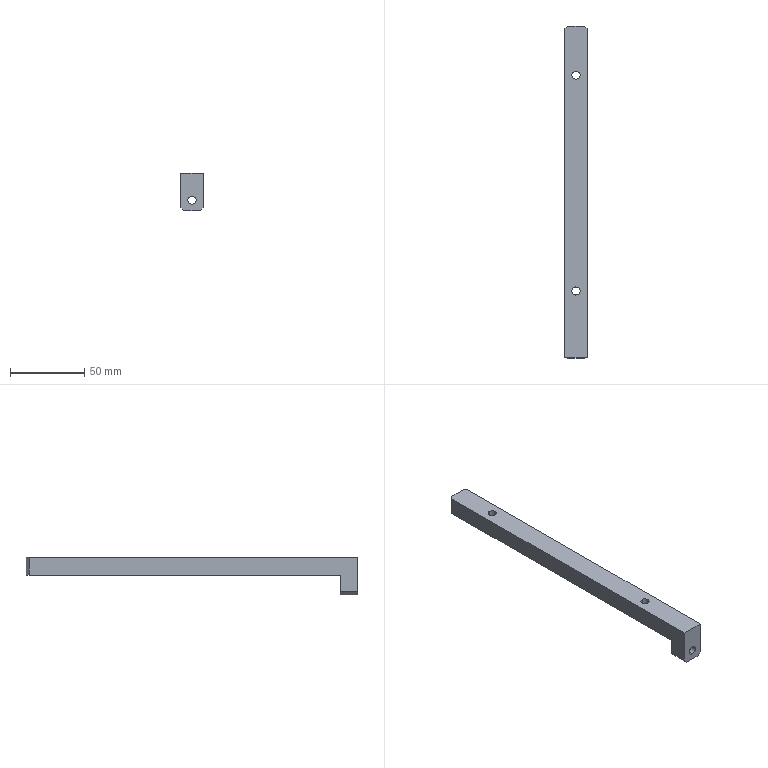Part | SolidWorks | features HoleWzd 2, Chamfer 1, Extrusion 1 | 1 solid | 24 faces | box 15 x 223.1 x 25 mm | volume 40922 mm3 | plane 14 | cylinder 10 | commonest cylinder face diameters 5.5 x6 10 x4
STEP:
#1=CARTESIAN_POINT('',(7.5,12.,-15.25));
#2=VERTEX_POINT('',#1);
#3=CARTESIAN_POINT('',(7.5,12.,-20.75));
#4=VERTEX_POINT('',#3);
#5=CARTESIAN_POINT('',(7.5,12.,-18.));
#6=DIRECTION('',(0.,-1.,0.));
#7=DIRECTION('',(0.,0.,-1.));
#8=AXIS2_PLACEMENT_3D('',#5,#6,#7);
#9=CIRCLE('',#8,2.75);
#10=EDGE_CURVE('',#2,#4,#9,.T.);
#11=ORIENTED_EDGE('',*,*,#10,.F.);
#12=CARTESIAN_POINT('',(7.5,0.,-15.25));
#13=VERTEX_POINT('',#12);
#14=CARTESIAN_POINT('',(7.5,0.,-15.25));
#15=DIRECTION('',(0.,-1.,0.));
#16=VECTOR('',#15,1000.);
#17=LINE('',#14,#16);
#18=EDGE_CURVE('',#2,#13,#17,.T.);
#19=ORIENTED_EDGE('',*,*,#18,.T.);
#20=CARTESIAN_POINT('',(7.5,0.,-20.75));
#21=VERTEX_POINT('',#20);
#22=CARTESIAN_POINT('',(7.5,0.,-18.));
#23=DIRECTION('',(0.,-1.,0.));
#24=DIRECTION('',(0.,0.,-1.));
#25=AXIS2_PLACEMENT_3D('',#22,#23,#24);
#26=CIRCLE('',#25,2.75);
#27=EDGE_CURVE('',#13,#21,#26,.T.);
#28=ORIENTED_EDGE('',*,*,#27,.T.);
#29=CARTESIAN_POINT('',(7.5,0.,-20.75));
#30=DIRECTION('',(0.,-1.,0.));
#31=VECTOR('',#30,1000.);
#32=LINE('',#29,#31);
#33=EDGE_CURVE('',#4,#21,#32,.T.);
#34=ORIENTED_EDGE('',*,*,#33,.F.);
#35=EDGE_LOOP('',(#11,#19,#28,#34));
#36=FACE_OUTER_BOUND('',#35,.T.);
#37=CARTESIAN_POINT('',(7.5,0.,-18.));
#38=DIRECTION('',(0.,-1.,0.));
#39=DIRECTION('',(0.,0.,-1.));
#40=AXIS2_PLACEMENT_3D('',#37,#38,#39);
#41=CYLINDRICAL_SURFACE('',#40,2.75);
#42=ADVANCED_FACE('',(#36),#41,.F.);
#43=CARTESIAN_POINT('',(7.5,185.,-6.3));
#44=VERTEX_POINT('',#43);
#45=CARTESIAN_POINT('',(7.5,195.,-6.3));
#46=VERTEX_POINT('',#45);
#47=CARTESIAN_POINT('',(7.5,190.,-6.3));
#48=DIRECTION('',(0.,0.,-1.));
#49=DIRECTION('',(0.,1.,0.));
#50=AXIS2_PLACEMENT_3D('',#47,#48,#49);
#51=CIRCLE('',#50,5.);
#52=EDGE_CURVE('',#44,#46,#51,.T.);
#53=ORIENTED_EDGE('',*,*,#52,.F.);
#54=CARTESIAN_POINT('',(7.5,185.,-12.));
#55=VERTEX_POINT('',#54);
#56=CARTESIAN_POINT('',(7.5,185.,-12.));
#57=DIRECTION('',(0.,0.,-1.));
#58=VECTOR('',#57,1000.);
#59=LINE('',#56,#58);
#60=EDGE_CURVE('',#44,#55,#59,.T.);
#61=ORIENTED_EDGE('',*,*,#60,.T.);
#62=CARTESIAN_POINT('',(7.5,195.,-12.));
#63=VERTEX_POINT('',#62);
#64=CARTESIAN_POINT('',(7.5,190.,-12.));
#65=DIRECTION('',(0.,0.,-1.));
#66=DIRECTION('',(0.,1.,0.));
#67=AXIS2_PLACEMENT_3D('',#64,#65,#66);
#68=CIRCLE('',#67,5.);
#69=EDGE_CURVE('',#55,#63,#68,.T.);
#70=ORIENTED_EDGE('',*,*,#69,.T.);
#71=CARTESIAN_POINT('',(7.5,195.,-12.));
#72=DIRECTION('',(0.,0.,-1.));
#73=VECTOR('',#72,1000.);
#74=LINE('',#71,#73);
#75=EDGE_CURVE('',#46,#63,#74,.T.);
#76=ORIENTED_EDGE('',*,*,#75,.F.);
#77=EDGE_LOOP('',(#53,#61,#70,#76));
#78=FACE_OUTER_BOUND('',#77,.T.);
#79=CARTESIAN_POINT('',(7.5,190.,-12.));
#80=DIRECTION('',(0.,0.,-1.));
#81=DIRECTION('',(0.,1.,0.));
#82=AXIS2_PLACEMENT_3D('',#79,#80,#81);
#83=CYLINDRICAL_SURFACE('',#82,5.);
#84=ADVANCED_FACE('',(#78),#83,.F.);
#85=CARTESIAN_POINT('',(7.5,187.25,0.));
#86=VERTEX_POINT('',#85);
#87=CARTESIAN_POINT('',(7.5,192.75,0.));
#88=VERTEX_POINT('',#87);
#89=CARTESIAN_POINT('',(7.5,190.,0.));
#90=DIRECTION('',(0.,0.,-1.));
#91=DIRECTION('',(0.,1.,0.));
#92=AXIS2_PLACEMENT_3D('',#89,#90,#91);
#93=CIRCLE('',#92,2.75);
#94=EDGE_CURVE('',#86,#88,#93,.T.);
#95=ORIENTED_EDGE('',*,*,#94,.F.);
#96=CARTESIAN_POINT('',(7.5,187.25,-6.3));
#97=VERTEX_POINT('',#96);
#98=CARTESIAN_POINT('',(7.5,187.25,-12.));
#99=DIRECTION('',(0.,0.,-1.));
#100=VECTOR('',#99,1000.);
#101=LINE('',#98,#100);
#102=EDGE_CURVE('',#86,#97,#101,.T.);
#103=ORIENTED_EDGE('',*,*,#102,.T.);
#104=CARTESIAN_POINT('',(7.5,192.75,-6.3));
#105=VERTEX_POINT('',#104);
#106=CARTESIAN_POINT('',(7.5,190.,-6.3));
#107=DIRECTION('',(0.,0.,-1.));
#108=DIRECTION('',(0.,1.,0.));
#109=AXIS2_PLACEMENT_3D('',#106,#107,#108);
#110=CIRCLE('',#109,2.75);
#111=EDGE_CURVE('',#97,#105,#110,.T.);
#112=ORIENTED_EDGE('',*,*,#111,.T.);
#113=CARTESIAN_POINT('',(7.5,192.75,-12.));
#114=DIRECTION('',(0.,0.,-1.));
#115=VECTOR('',#114,1000.);
#116=LINE('',#113,#115);
#117=EDGE_CURVE('',#88,#105,#116,.T.);
#118=ORIENTED_EDGE('',*,*,#117,.F.);
#119=EDGE_LOOP('',(#95,#103,#112,#118));
#120=FACE_OUTER_BOUND('',#119,.T.);
#121=CARTESIAN_POINT('',(7.5,190.,-12.));
#122=DIRECTION('',(0.,0.,-1.));
#123=DIRECTION('',(0.,1.,0.));
#124=AXIS2_PLACEMENT_3D('',#121,#122,#123);
#125=CYLINDRICAL_SURFACE('',#124,2.75);
#126=ADVANCED_FACE('',(#120),#125,.F.);
#127=CARTESIAN_POINT('',(7.5,40.,-6.3));
#128=VERTEX_POINT('',#127);
#129=CARTESIAN_POINT('',(7.5,50.,-6.3));
#130=VERTEX_POINT('',#129);
#131=CARTESIAN_POINT('',(7.5,45.,-6.3));
#132=DIRECTION('',(0.,0.,-1.));
#133=DIRECTION('',(0.,1.,0.));
#134=AXIS2_PLACEMENT_3D('',#131,#132,#133);
#135=CIRCLE('',#134,5.);
#136=EDGE_CURVE('',#128,#130,#135,.T.);
#137=ORIENTED_EDGE('',*,*,#136,.F.);
#138=CARTESIAN_POINT('',(7.5,40.,-12.));
#139=VERTEX_POINT('',#138);
#140=CARTESIAN_POINT('',(7.5,40.,-12.));
#141=DIRECTION('',(0.,0.,-1.));
#142=VECTOR('',#141,1000.);
#143=LINE('',#140,#142);
#144=EDGE_CURVE('',#128,#139,#143,.T.);
#145=ORIENTED_EDGE('',*,*,#144,.T.);
#146=CARTESIAN_POINT('',(7.5,50.,-12.));
#147=VERTEX_POINT('',#146);
#148=CARTESIAN_POINT('',(7.5,45.,-12.));
#149=DIRECTION('',(0.,0.,-1.));
#150=DIRECTION('',(0.,1.,0.));
#151=AXIS2_PLACEMENT_3D('',#148,#149,#150);
#152=CIRCLE('',#151,5.);
#153=EDGE_CURVE('',#139,#147,#152,.T.);
#154=ORIENTED_EDGE('',*,*,#153,.T.);
#155=CARTESIAN_POINT('',(7.5,50.,-12.));
#156=DIRECTION('',(0.,0.,-1.));
#157=VECTOR('',#156,1000.);
#158=LINE('',#155,#157);
#159=EDGE_CURVE('',#130,#147,#158,.T.);
#160=ORIENTED_EDGE('',*,*,#159,.F.);
#161=EDGE_LOOP('',(#137,#145,#154,#160));
#162=FACE_OUTER_BOUND('',#161,.T.);
#163=CARTESIAN_POINT('',(7.5,45.,-12.));
#164=DIRECTION('',(0.,0.,-1.));
#165=DIRECTION('',(0.,1.,0.));
#166=AXIS2_PLACEMENT_3D('',#163,#164,#165);
#167=CYLINDRICAL_SURFACE('',#166,5.);
#168=ADVANCED_FACE('',(#162),#167,.F.);
#169=CARTESIAN_POINT('',(7.5,42.25,0.));
#170=VERTEX_POINT('',#169);
#171=CARTESIAN_POINT('',(7.5,47.75,0.));
#172=VERTEX_POINT('',#171);
#173=CARTESIAN_POINT('',(7.5,45.,0.));
#174=DIRECTION('',(0.,0.,-1.));
#175=DIRECTION('',(0.,1.,0.));
#176=AXIS2_PLACEMENT_3D('',#173,#174,#175);
#177=CIRCLE('',#176,2.75);
#178=EDGE_CURVE('',#170,#172,#177,.T.);
#179=ORIENTED_EDGE('',*,*,#178,.F.);
#180=CARTESIAN_POINT('',(7.5,42.25,-6.3));
#181=VERTEX_POINT('',#180);
#182=CARTESIAN_POINT('',(7.5,42.25,-12.));
#183=DIRECTION('',(0.,0.,-1.));
#184=VECTOR('',#183,1000.);
#185=LINE('',#182,#184);
#186=EDGE_CURVE('',#170,#181,#185,.T.);
#187=ORIENTED_EDGE('',*,*,#186,.T.);
#188=CARTESIAN_POINT('',(7.5,47.75,-6.3));
#189=VERTEX_POINT('',#188);
#190=CARTESIAN_POINT('',(7.5,45.,-6.3));
#191=DIRECTION('',(0.,0.,-1.));
#192=DIRECTION('',(0.,1.,0.));
#193=AXIS2_PLACEMENT_3D('',#190,#191,#192);
#194=CIRCLE('',#193,2.75);
#195=EDGE_CURVE('',#181,#189,#194,.T.);
#196=ORIENTED_EDGE('',*,*,#195,.T.);
#197=CARTESIAN_POINT('',(7.5,47.75,-12.));
#198=DIRECTION('',(0.,0.,-1.));
#199=VECTOR('',#198,1000.);
#200=LINE('',#197,#199);
#201=EDGE_CURVE('',#172,#189,#200,.T.);
#202=ORIENTED_EDGE('',*,*,#201,.F.);
#203=EDGE_LOOP('',(#179,#187,#196,#202));
#204=FACE_OUTER_BOUND('',#203,.T.);
#205=CARTESIAN_POINT('',(7.5,45.,-12.));
#206=DIRECTION('',(0.,0.,-1.));
#207=DIRECTION('',(0.,1.,0.));
#208=AXIS2_PLACEMENT_3D('',#205,#206,#207);
#209=CYLINDRICAL_SURFACE('',#208,2.75);
#210=ADVANCED_FACE('',(#204),#209,.F.);
#211=CARTESIAN_POINT('',(7.5,190.,0.));
#212=DIRECTION('',(0.,0.,-1.));
#213=DIRECTION('',(0.,1.,0.));
#214=AXIS2_PLACEMENT_3D('',#211,#212,#213);
#215=CIRCLE('',#214,2.75);
#216=EDGE_CURVE('',#88,#86,#215,.T.);
#217=ORIENTED_EDGE('',*,*,#216,.T.);
#218=ORIENTED_EDGE('',*,*,#94,.T.);
#219=EDGE_LOOP('',(#217,#218));
#220=FACE_BOUND('',#219,.T.);
#221=CARTESIAN_POINT('',(7.5,45.,0.));
#222=DIRECTION('',(0.,0.,-1.));
#223=DIRECTION('',(0.,1.,0.));
#224=AXIS2_PLACEMENT_3D('',#221,#222,#223);
#225=CIRCLE('',#224,2.75);
#226=EDGE_CURVE('',#172,#170,#225,.T.);
#227=ORIENTED_EDGE('',*,*,#226,.T.);
#228=ORIENTED_EDGE('',*,*,#178,.T.);
#229=EDGE_LOOP('',(#227,#228));
#230=FACE_BOUND('',#229,.T.);
#231=CARTESIAN_POINT('',(13.,223.1,0.));
#232=VERTEX_POINT('',#231);
#233=CARTESIAN_POINT('',(2.,223.1,0.));
#234=VERTEX_POINT('',#233);
#235=CARTESIAN_POINT('',(15.,223.1,0.));
#236=DIRECTION('',(-1.,0.,0.));
#237=VECTOR('',#236,1000.);
#238=LINE('',#235,#237);
#239=EDGE_CURVE('',#232,#234,#238,.T.);
#240=ORIENTED_EDGE('',*,*,#239,.T.);
#241=CARTESIAN_POINT('',(0.,221.1,0.));
#242=VERTEX_POINT('',#241);
#243=CARTESIAN_POINT('',(2.,223.1,0.));
#244=DIRECTION('',(-0.7071,-0.7071,0.));
#245=VECTOR('',#244,1000.);
#246=LINE('',#243,#245);
#247=EDGE_CURVE('',#234,#242,#246,.T.);
#248=ORIENTED_EDGE('',*,*,#247,.T.);
#249=CARTESIAN_POINT('',(0.,0.,0.));
#250=VERTEX_POINT('',#249);
#251=CARTESIAN_POINT('',(0.,223.1,0.));
#252=DIRECTION('',(0.,-1.,0.));
#253=VECTOR('',#252,1000.);
#254=LINE('',#251,#253);
#255=EDGE_CURVE('',#242,#250,#254,.T.);
#256=ORIENTED_EDGE('',*,*,#255,.T.);
#257=CARTESIAN_POINT('',(15.,0.,0.));
#258=VERTEX_POINT('',#257);
#259=CARTESIAN_POINT('',(15.,0.,0.));
#260=DIRECTION('',(-1.,0.,0.));
#261=VECTOR('',#260,1000.);
#262=LINE('',#259,#261);
#263=EDGE_CURVE('',#258,#250,#262,.T.);
#264=ORIENTED_EDGE('',*,*,#263,.F.);
#265=CARTESIAN_POINT('',(15.,221.1,0.));
#266=VERTEX_POINT('',#265);
#267=CARTESIAN_POINT('',(15.,223.1,0.));
#268=DIRECTION('',(0.,-1.,0.));
#269=VECTOR('',#268,1000.);
#270=LINE('',#267,#269);
#271=EDGE_CURVE('',#266,#258,#270,.T.);
#272=ORIENTED_EDGE('',*,*,#271,.F.);
#273=CARTESIAN_POINT('',(15.,221.1,0.));
#274=DIRECTION('',(-0.7071,0.7071,0.));
#275=VECTOR('',#274,1000.);
#276=LINE('',#273,#275);
#277=EDGE_CURVE('',#266,#232,#276,.T.);
#278=ORIENTED_EDGE('',*,*,#277,.T.);
#279=EDGE_LOOP('',(#240,#248,#256,#264,#272,#278));
#280=FACE_OUTER_BOUND('',#279,.T.);
#281=CARTESIAN_POINT('',(15.,223.1,0.));
#282=DIRECTION('',(0.,0.,-1.));
#283=DIRECTION('',(-1.,0.,0.));
#284=AXIS2_PLACEMENT_3D('',#281,#282,#283);
#285=PLANE('',#284);
#286=ADVANCED_FACE('',(#220,#230,#280),#285,.F.);
#287=CARTESIAN_POINT('',(7.5,0.,-18.));
#288=DIRECTION('',(0.,-1.,0.));
#289=DIRECTION('',(0.,0.,-1.));
#290=AXIS2_PLACEMENT_3D('',#287,#288,#289);
#291=CIRCLE('',#290,2.75);
#292=EDGE_CURVE('',#21,#13,#291,.T.);
#293=ORIENTED_EDGE('',*,*,#292,.F.);
#294=ORIENTED_EDGE('',*,*,#27,.F.);
#295=EDGE_LOOP('',(#293,#294));
#296=FACE_BOUND('',#295,.T.);
#297=CARTESIAN_POINT('',(0.,0.,-23.));
#298=VERTEX_POINT('',#297);
#299=CARTESIAN_POINT('',(0.,0.,0.));
#300=DIRECTION('',(0.,0.,-1.));
#301=VECTOR('',#300,1000.);
#302=LINE('',#299,#301);
#303=EDGE_CURVE('',#250,#298,#302,.T.);
#304=ORIENTED_EDGE('',*,*,#303,.T.);
#305=CARTESIAN_POINT('',(2.,0.,-25.));
#306=VERTEX_POINT('',#305);
#307=CARTESIAN_POINT('',(2.,0.,-25.));
#308=DIRECTION('',(0.7071,0.,-0.7071));
#309=VECTOR('',#308,1000.);
#310=LINE('',#307,#309);
#311=EDGE_CURVE('',#298,#306,#310,.T.);
#312=ORIENTED_EDGE('',*,*,#311,.T.);
#313=CARTESIAN_POINT('',(13.,0.,-25.));
#314=VERTEX_POINT('',#313);
#315=CARTESIAN_POINT('',(15.,0.,-25.));
#316=DIRECTION('',(-1.,0.,0.));
#317=VECTOR('',#316,1000.);
#318=LINE('',#315,#317);
#319=EDGE_CURVE('',#314,#306,#318,.T.);
#320=ORIENTED_EDGE('',*,*,#319,.F.);
#321=CARTESIAN_POINT('',(15.,0.,-23.));
#322=VERTEX_POINT('',#321);
#323=CARTESIAN_POINT('',(15.,0.,-23.));
#324=DIRECTION('',(0.7071,0.,0.7071));
#325=VECTOR('',#324,1000.);
#326=LINE('',#323,#325);
#327=EDGE_CURVE('',#314,#322,#326,.T.);
#328=ORIENTED_EDGE('',*,*,#327,.T.);
#329=CARTESIAN_POINT('',(15.,0.,0.));
#330=DIRECTION('',(0.,0.,-1.));
#331=VECTOR('',#330,1000.);
#332=LINE('',#329,#331);
#333=EDGE_CURVE('',#258,#322,#332,.T.);
#334=ORIENTED_EDGE('',*,*,#333,.F.);
#335=ORIENTED_EDGE('',*,*,#263,.T.);
#336=EDGE_LOOP('',(#304,#312,#320,#328,#334,#335));
#337=FACE_OUTER_BOUND('',#336,.T.);
#338=CARTESIAN_POINT('',(15.,0.,0.));
#339=DIRECTION('',(0.,1.,0.));
#340=DIRECTION('',(0.,0.,1.));
#341=AXIS2_PLACEMENT_3D('',#338,#339,#340);
#342=PLANE('',#341);
#343=ADVANCED_FACE('',(#296,#337),#342,.F.);
#344=ORIENTED_EDGE('',*,*,#319,.T.);
#345=CARTESIAN_POINT('',(2.,12.,-25.));
#346=VERTEX_POINT('',#345);
#347=CARTESIAN_POINT('',(2.,0.,-25.));
#348=DIRECTION('',(0.,1.,0.));
#349=VECTOR('',#348,1000.);
#350=LINE('',#347,#349);
#351=EDGE_CURVE('',#306,#346,#350,.T.);
#352=ORIENTED_EDGE('',*,*,#351,.T.);
#353=CARTESIAN_POINT('',(13.,12.,-25.));
#354=VERTEX_POINT('',#353);
#355=CARTESIAN_POINT('',(15.,12.,-25.));
#356=DIRECTION('',(-1.,0.,0.));
#357=VECTOR('',#356,1000.);
#358=LINE('',#355,#357);
#359=EDGE_CURVE('',#354,#346,#358,.T.);
#360=ORIENTED_EDGE('',*,*,#359,.F.);
#361=CARTESIAN_POINT('',(13.,0.,-25.));
#362=DIRECTION('',(0.,-1.,0.));
#363=VECTOR('',#362,1000.);
#364=LINE('',#361,#363);
#365=EDGE_CURVE('',#354,#314,#364,.T.);
#366=ORIENTED_EDGE('',*,*,#365,.T.);
#367=EDGE_LOOP('',(#344,#352,#360,#366));
#368=FACE_OUTER_BOUND('',#367,.T.);
#369=CARTESIAN_POINT('',(15.,0.,-25.));
#370=DIRECTION('',(0.,0.,1.));
#371=DIRECTION('',(1.,0.,0.));
#372=AXIS2_PLACEMENT_3D('',#369,#370,#371);
#373=PLANE('',#372);
#374=ADVANCED_FACE('',(#368),#373,.F.);
#375=CARTESIAN_POINT('',(7.5,12.,-18.));
#376=DIRECTION('',(0.,-1.,0.));
#377=DIRECTION('',(0.,0.,-1.));
#378=AXIS2_PLACEMENT_3D('',#375,#376,#377);
#379=CIRCLE('',#378,2.75);
#380=EDGE_CURVE('',#4,#2,#379,.T.);
#381=ORIENTED_EDGE('',*,*,#380,.T.);
#382=ORIENTED_EDGE('',*,*,#10,.T.);
#383=EDGE_LOOP('',(#381,#382));
#384=FACE_BOUND('',#383,.T.);
#385=ORIENTED_EDGE('',*,*,#359,.T.);
#386=CARTESIAN_POINT('',(0.,12.,-23.));
#387=VERTEX_POINT('',#386);
#388=CARTESIAN_POINT('',(2.,12.,-25.));
#389=DIRECTION('',(-0.7071,0.,0.7071));
#390=VECTOR('',#389,1000.);
#391=LINE('',#388,#390);
#392=EDGE_CURVE('',#346,#387,#391,.T.);
#393=ORIENTED_EDGE('',*,*,#392,.T.);
#394=CARTESIAN_POINT('',(0.,12.,-12.));
#395=VERTEX_POINT('',#394);
#396=CARTESIAN_POINT('',(0.,12.,-25.));
#397=DIRECTION('',(0.,0.,1.));
#398=VECTOR('',#397,1000.);
#399=LINE('',#396,#398);
#400=EDGE_CURVE('',#387,#395,#399,.T.);
#401=ORIENTED_EDGE('',*,*,#400,.T.);
#402=CARTESIAN_POINT('',(15.,12.,-12.));
#403=VERTEX_POINT('',#402);
#404=CARTESIAN_POINT('',(15.,12.,-12.));
#405=DIRECTION('',(-1.,0.,0.));
#406=VECTOR('',#405,1000.);
#407=LINE('',#404,#406);
#408=EDGE_CURVE('',#403,#395,#407,.T.);
#409=ORIENTED_EDGE('',*,*,#408,.F.);
#410=CARTESIAN_POINT('',(15.,12.,-23.));
#411=VERTEX_POINT('',#410);
#412=CARTESIAN_POINT('',(15.,12.,-25.));
#413=DIRECTION('',(0.,0.,1.));
#414=VECTOR('',#413,1000.);
#415=LINE('',#412,#414);
#416=EDGE_CURVE('',#411,#403,#415,.T.);
#417=ORIENTED_EDGE('',*,*,#416,.F.);
#418=CARTESIAN_POINT('',(15.,12.,-23.));
#419=DIRECTION('',(-0.7071,0.,-0.7071));
#420=VECTOR('',#419,1000.);
#421=LINE('',#418,#420);
#422=EDGE_CURVE('',#411,#354,#421,.T.);
#423=ORIENTED_EDGE('',*,*,#422,.T.);
#424=EDGE_LOOP('',(#385,#393,#401,#409,#417,#423));
#425=FACE_OUTER_BOUND('',#424,.T.);
#426=CARTESIAN_POINT('',(15.,12.,-25.));
#427=DIRECTION('',(0.,-1.,0.));
#428=DIRECTION('',(0.,0.,-1.));
#429=AXIS2_PLACEMENT_3D('',#426,#427,#428);
#430=PLANE('',#429);
#431=ADVANCED_FACE('',(#384,#425),#430,.F.);
#432=CARTESIAN_POINT('',(7.5,190.,-12.));
#433=DIRECTION('',(0.,0.,-1.));
#434=DIRECTION('',(0.,1.,0.));
#435=AXIS2_PLACEMENT_3D('',#432,#433,#434);
#436=CIRCLE('',#435,5.);
#437=EDGE_CURVE('',#63,#55,#436,.T.);
#438=ORIENTED_EDGE('',*,*,#437,.F.);
#439=ORIENTED_EDGE('',*,*,#69,.F.);
#440=EDGE_LOOP('',(#438,#439));
#441=FACE_BOUND('',#440,.T.);
#442=CARTESIAN_POINT('',(7.5,45.,-12.));
#443=DIRECTION('',(0.,0.,-1.));
#444=DIRECTION('',(0.,1.,0.));
#445=AXIS2_PLACEMENT_3D('',#442,#443,#444);
#446=CIRCLE('',#445,5.);
#447=EDGE_CURVE('',#147,#139,#446,.T.);
#448=ORIENTED_EDGE('',*,*,#447,.F.);
#449=ORIENTED_EDGE('',*,*,#153,.F.);
#450=EDGE_LOOP('',(#448,#449));
#451=FACE_BOUND('',#450,.T.);
#452=CARTESIAN_POINT('',(0.,221.1,-12.));
#453=VERTEX_POINT('',#452);
#454=CARTESIAN_POINT('',(0.,12.,-12.));
#455=DIRECTION('',(0.,1.,0.));
#456=VECTOR('',#455,1000.);
#457=LINE('',#454,#456);
#458=EDGE_CURVE('',#395,#453,#457,.T.);
#459=ORIENTED_EDGE('',*,*,#458,.T.);
#460=CARTESIAN_POINT('',(2.,223.1,-12.));
#461=VERTEX_POINT('',#460);
#462=CARTESIAN_POINT('',(2.,223.1,-12.));
#463=DIRECTION('',(0.7071,0.7071,0.));
#464=VECTOR('',#463,1000.);
#465=LINE('',#462,#464);
#466=EDGE_CURVE('',#453,#461,#465,.T.);
#467=ORIENTED_EDGE('',*,*,#466,.T.);
#468=CARTESIAN_POINT('',(13.,223.1,-12.));
#469=VERTEX_POINT('',#468);
#470=CARTESIAN_POINT('',(15.,223.1,-12.));
#471=DIRECTION('',(-1.,0.,0.));
#472=VECTOR('',#471,1000.);
#473=LINE('',#470,#472);
#474=EDGE_CURVE('',#469,#461,#473,.T.);
#475=ORIENTED_EDGE('',*,*,#474,.F.);
#476=CARTESIAN_POINT('',(15.,221.1,-12.));
#477=VERTEX_POINT('',#476);
#478=CARTESIAN_POINT('',(15.,221.1,-12.));
#479=DIRECTION('',(0.7071,-0.7071,0.));
#480=VECTOR('',#479,1000.);
#481=LINE('',#478,#480);
#482=EDGE_CURVE('',#469,#477,#481,.T.);
#483=ORIENTED_EDGE('',*,*,#482,.T.);
#484=CARTESIAN_POINT('',(15.,12.,-12.));
#485=DIRECTION('',(0.,1.,0.));
#486=VECTOR('',#485,1000.);
#487=LINE('',#484,#486);
#488=EDGE_CURVE('',#403,#477,#487,.T.);
#489=ORIENTED_EDGE('',*,*,#488,.F.);
#490=ORIENTED_EDGE('',*,*,#408,.T.);
#491=EDGE_LOOP('',(#459,#467,#475,#483,#489,#490));
#492=FACE_OUTER_BOUND('',#491,.T.);
#493=CARTESIAN_POINT('',(15.,12.,-12.));
#494=DIRECTION('',(0.,0.,1.));
#495=DIRECTION('',(0.,-1.,0.));
#496=AXIS2_PLACEMENT_3D('',#493,#494,#495);
#497=PLANE('',#496);
#498=ADVANCED_FACE('',(#441,#451,#492),#497,.F.);
#499=ORIENTED_EDGE('',*,*,#474,.T.);
#500=CARTESIAN_POINT('',(2.,223.1,-12.));
#501=DIRECTION('',(0.,0.,1.));
#502=VECTOR('',#501,1000.);
#503=LINE('',#500,#502);
#504=EDGE_CURVE('',#461,#234,#503,.T.);
#505=ORIENTED_EDGE('',*,*,#504,.T.);
#506=ORIENTED_EDGE('',*,*,#239,.F.);
#507=CARTESIAN_POINT('',(13.,223.1,-12.));
#508=DIRECTION('',(0.,0.,-1.));
#509=VECTOR('',#508,1000.);
#510=LINE('',#507,#509);
#511=EDGE_CURVE('',#232,#469,#510,.T.);
#512=ORIENTED_EDGE('',*,*,#511,.T.);
#513=EDGE_LOOP('',(#499,#505,#506,#512));
#514=FACE_OUTER_BOUND('',#513,.T.);
#515=CARTESIAN_POINT('',(15.,223.1,-12.));
#516=DIRECTION('',(0.,-1.,0.));
#517=DIRECTION('',(0.,0.,-1.));
#518=AXIS2_PLACEMENT_3D('',#515,#516,#517);
#519=PLANE('',#518);
#520=ADVANCED_FACE('',(#514),#519,.F.);
#521=ORIENTED_EDGE('',*,*,#333,.T.);
#522=CARTESIAN_POINT('',(15.,12.,-23.));
#523=DIRECTION('',(0.,1.,0.));
#524=VECTOR('',#523,1000.);
#525=LINE('',#522,#524);
#526=EDGE_CURVE('',#322,#411,#525,.T.);
#527=ORIENTED_EDGE('',*,*,#526,.T.);
#528=ORIENTED_EDGE('',*,*,#416,.T.);
#529=ORIENTED_EDGE('',*,*,#488,.T.);
#530=CARTESIAN_POINT('',(15.,221.1,0.));
#531=DIRECTION('',(0.,0.,1.));
#532=VECTOR('',#531,1000.);
#533=LINE('',#530,#532);
#534=EDGE_CURVE('',#477,#266,#533,.T.);
#535=ORIENTED_EDGE('',*,*,#534,.T.);
#536=ORIENTED_EDGE('',*,*,#271,.T.);
#537=EDGE_LOOP('',(#521,#527,#528,#529,#535,#536));
#538=FACE_OUTER_BOUND('',#537,.T.);
#539=CARTESIAN_POINT('',(15.,0.,0.));
#540=DIRECTION('',(1.,0.,0.));
#541=DIRECTION('',(0.,0.,-1.));
#542=AXIS2_PLACEMENT_3D('',#539,#540,#541);
#543=PLANE('',#542);
#544=ADVANCED_FACE('',(#538),#543,.T.);
#545=ORIENTED_EDGE('',*,*,#400,.F.);
#546=CARTESIAN_POINT('',(0.,0.,-23.));
#547=DIRECTION('',(0.,-1.,0.));
#548=VECTOR('',#547,1000.);
#549=LINE('',#546,#548);
#550=EDGE_CURVE('',#387,#298,#549,.T.);
#551=ORIENTED_EDGE('',*,*,#550,.T.);
#552=ORIENTED_EDGE('',*,*,#303,.F.);
#553=ORIENTED_EDGE('',*,*,#255,.F.);
#554=CARTESIAN_POINT('',(0.,221.1,0.));
#555=DIRECTION('',(0.,0.,-1.));
#556=VECTOR('',#555,1000.);
#557=LINE('',#554,#556);
#558=EDGE_CURVE('',#242,#453,#557,.T.);
#559=ORIENTED_EDGE('',*,*,#558,.T.);
#560=ORIENTED_EDGE('',*,*,#458,.F.);
#561=EDGE_LOOP('',(#545,#551,#552,#553,#559,#560));
#562=FACE_OUTER_BOUND('',#561,.T.);
#563=CARTESIAN_POINT('',(0.,0.,0.));
#564=DIRECTION('',(1.,0.,0.));
#565=DIRECTION('',(0.,0.,-1.));
#566=AXIS2_PLACEMENT_3D('',#563,#564,#565);
#567=PLANE('',#566);
#568=ADVANCED_FACE('',(#562),#567,.F.);
#569=ORIENTED_EDGE('',*,*,#186,.F.);
#570=ORIENTED_EDGE('',*,*,#226,.F.);
#571=ORIENTED_EDGE('',*,*,#201,.T.);
#572=CARTESIAN_POINT('',(7.5,45.,-6.3));
#573=DIRECTION('',(0.,0.,-1.));
#574=DIRECTION('',(0.,1.,0.));
#575=AXIS2_PLACEMENT_3D('',#572,#573,#574);
#576=CIRCLE('',#575,2.75);
#577=EDGE_CURVE('',#189,#181,#576,.T.);
#578=ORIENTED_EDGE('',*,*,#577,.T.);
#579=EDGE_LOOP('',(#569,#570,#571,#578));
#580=FACE_OUTER_BOUND('',#579,.T.);
#581=CARTESIAN_POINT('',(7.5,45.,-12.));
#582=DIRECTION('',(0.,0.,-1.));
#583=DIRECTION('',(0.,1.,0.));
#584=AXIS2_PLACEMENT_3D('',#581,#582,#583);
#585=CYLINDRICAL_SURFACE('',#584,2.75);
#586=ADVANCED_FACE('',(#580),#585,.F.);
#587=ORIENTED_EDGE('',*,*,#577,.F.);
#588=ORIENTED_EDGE('',*,*,#195,.F.);
#589=EDGE_LOOP('',(#587,#588));
#590=FACE_BOUND('',#589,.T.);
#591=CARTESIAN_POINT('',(7.5,45.,-6.3));
#592=DIRECTION('',(0.,0.,-1.));
#593=DIRECTION('',(0.,1.,0.));
#594=AXIS2_PLACEMENT_3D('',#591,#592,#593);
#595=CIRCLE('',#594,5.);
#596=EDGE_CURVE('',#130,#128,#595,.T.);
#597=ORIENTED_EDGE('',*,*,#596,.T.);
#598=ORIENTED_EDGE('',*,*,#136,.T.);
#599=EDGE_LOOP('',(#597,#598));
#600=FACE_OUTER_BOUND('',#599,.T.);
#601=CARTESIAN_POINT('',(10.25,45.,-6.3));
#602=DIRECTION('',(0.,0.,1.));
#603=DIRECTION('',(0.,-1.,0.));
#604=AXIS2_PLACEMENT_3D('',#601,#602,#603);
#605=PLANE('',#604);
#606=ADVANCED_FACE('',(#590,#600),#605,.F.);
#607=ORIENTED_EDGE('',*,*,#144,.F.);
#608=ORIENTED_EDGE('',*,*,#596,.F.);
#609=ORIENTED_EDGE('',*,*,#159,.T.);
#610=ORIENTED_EDGE('',*,*,#447,.T.);
#611=EDGE_LOOP('',(#607,#608,#609,#610));
#612=FACE_OUTER_BOUND('',#611,.T.);
#613=CARTESIAN_POINT('',(7.5,45.,-12.));
#614=DIRECTION('',(0.,0.,-1.));
#615=DIRECTION('',(0.,1.,0.));
#616=AXIS2_PLACEMENT_3D('',#613,#614,#615);
#617=CYLINDRICAL_SURFACE('',#616,5.);
#618=ADVANCED_FACE('',(#612),#617,.F.);
#619=ORIENTED_EDGE('',*,*,#102,.F.);
#620=ORIENTED_EDGE('',*,*,#216,.F.);
#621=ORIENTED_EDGE('',*,*,#117,.T.);
#622=CARTESIAN_POINT('',(7.5,190.,-6.3));
#623=DIRECTION('',(0.,0.,-1.));
#624=DIRECTION('',(0.,1.,0.));
#625=AXIS2_PLACEMENT_3D('',#622,#623,#624);
#626=CIRCLE('',#625,2.75);
#627=EDGE_CURVE('',#105,#97,#626,.T.);
#628=ORIENTED_EDGE('',*,*,#627,.T.);
#629=EDGE_LOOP('',(#619,#620,#621,#628));
#630=FACE_OUTER_BOUND('',#629,.T.);
#631=CARTESIAN_POINT('',(7.5,190.,-12.));
#632=DIRECTION('',(0.,0.,-1.));
#633=DIRECTION('',(0.,1.,0.));
#634=AXIS2_PLACEMENT_3D('',#631,#632,#633);
#635=CYLINDRICAL_SURFACE('',#634,2.75);
#636=ADVANCED_FACE('',(#630),#635,.F.);
#637=ORIENTED_EDGE('',*,*,#627,.F.);
#638=ORIENTED_EDGE('',*,*,#111,.F.);
#639=EDGE_LOOP('',(#637,#638));
#640=FACE_BOUND('',#639,.T.);
#641=CARTESIAN_POINT('',(7.5,190.,-6.3));
#642=DIRECTION('',(0.,0.,-1.));
#643=DIRECTION('',(0.,1.,0.));
#644=AXIS2_PLACEMENT_3D('',#641,#642,#643);
#645=CIRCLE('',#644,5.);
#646=EDGE_CURVE('',#46,#44,#645,.T.);
#647=ORIENTED_EDGE('',*,*,#646,.T.);
#648=ORIENTED_EDGE('',*,*,#52,.T.);
#649=EDGE_LOOP('',(#647,#648));
#650=FACE_OUTER_BOUND('',#649,.T.);
#651=CARTESIAN_POINT('',(10.25,190.,-6.3));
#652=DIRECTION('',(0.,0.,1.));
#653=DIRECTION('',(0.,-1.,0.));
#654=AXIS2_PLACEMENT_3D('',#651,#652,#653);
#655=PLANE('',#654);
#656=ADVANCED_FACE('',(#640,#650),#655,.F.);
#657=ORIENTED_EDGE('',*,*,#60,.F.);
#658=ORIENTED_EDGE('',*,*,#646,.F.);
#659=ORIENTED_EDGE('',*,*,#75,.T.);
#660=ORIENTED_EDGE('',*,*,#437,.T.);
#661=EDGE_LOOP('',(#657,#658,#659,#660));
#662=FACE_OUTER_BOUND('',#661,.T.);
#663=CARTESIAN_POINT('',(7.5,190.,-12.));
#664=DIRECTION('',(0.,0.,-1.));
#665=DIRECTION('',(0.,1.,0.));
#666=AXIS2_PLACEMENT_3D('',#663,#664,#665);
#667=CYLINDRICAL_SURFACE('',#666,5.);
#668=ADVANCED_FACE('',(#662),#667,.F.);
#669=ORIENTED_EDGE('',*,*,#18,.F.);
#670=ORIENTED_EDGE('',*,*,#380,.F.);
#671=ORIENTED_EDGE('',*,*,#33,.T.);
#672=ORIENTED_EDGE('',*,*,#292,.T.);
#673=EDGE_LOOP('',(#669,#670,#671,#672));
#674=FACE_OUTER_BOUND('',#673,.T.);
#675=CARTESIAN_POINT('',(7.5,0.,-18.));
#676=DIRECTION('',(0.,-1.,0.));
#677=DIRECTION('',(0.,0.,-1.));
#678=AXIS2_PLACEMENT_3D('',#675,#676,#677);
#679=CYLINDRICAL_SURFACE('',#678,2.75);
#680=ADVANCED_FACE('',(#674),#679,.F.);
#681=ORIENTED_EDGE('',*,*,#311,.F.);
#682=ORIENTED_EDGE('',*,*,#550,.F.);
#683=ORIENTED_EDGE('',*,*,#392,.F.);
#684=ORIENTED_EDGE('',*,*,#351,.F.);
#685=EDGE_LOOP('',(#681,#682,#683,#684));
#686=FACE_OUTER_BOUND('',#685,.T.);
#687=CARTESIAN_POINT('',(2.,0.,-25.));
#688=DIRECTION('',(0.7071,0.,0.7071));
#689=DIRECTION('',(0.,1.,0.));
#690=AXIS2_PLACEMENT_3D('',#687,#688,#689);
#691=PLANE('',#690);
#692=ADVANCED_FACE('',(#686),#691,.F.);
#693=ORIENTED_EDGE('',*,*,#327,.F.);
#694=ORIENTED_EDGE('',*,*,#365,.F.);
#695=ORIENTED_EDGE('',*,*,#422,.F.);
#696=ORIENTED_EDGE('',*,*,#526,.F.);
#697=EDGE_LOOP('',(#693,#694,#695,#696));
#698=FACE_OUTER_BOUND('',#697,.T.);
#699=CARTESIAN_POINT('',(15.,0.,-23.));
#700=DIRECTION('',(0.7071,0.,-0.7071));
#701=DIRECTION('',(0.,-1.,0.));
#702=AXIS2_PLACEMENT_3D('',#699,#700,#701);
#703=PLANE('',#702);
#704=ADVANCED_FACE('',(#698),#703,.T.);
#705=ORIENTED_EDGE('',*,*,#466,.F.);
#706=ORIENTED_EDGE('',*,*,#558,.F.);
#707=ORIENTED_EDGE('',*,*,#247,.F.);
#708=ORIENTED_EDGE('',*,*,#504,.F.);
#709=EDGE_LOOP('',(#705,#706,#707,#708));
#710=FACE_OUTER_BOUND('',#709,.T.);
#711=CARTESIAN_POINT('',(2.,223.1,-12.));
#712=DIRECTION('',(0.7071,-0.7071,0.));
#713=DIRECTION('',(0.,0.,1.));
#714=AXIS2_PLACEMENT_3D('',#711,#712,#713);
#715=PLANE('',#714);
#716=ADVANCED_FACE('',(#710),#715,.F.);
#717=ORIENTED_EDGE('',*,*,#482,.F.);
#718=ORIENTED_EDGE('',*,*,#511,.F.);
#719=ORIENTED_EDGE('',*,*,#277,.F.);
#720=ORIENTED_EDGE('',*,*,#534,.F.);
#721=EDGE_LOOP('',(#717,#718,#719,#720));
#722=FACE_OUTER_BOUND('',#721,.T.);
#723=CARTESIAN_POINT('',(15.,221.1,0.));
#724=DIRECTION('',(0.7071,0.7071,0.));
#725=DIRECTION('',(0.,0.,-1.));
#726=AXIS2_PLACEMENT_3D('',#723,#724,#725);
#727=PLANE('',#726);
#728=ADVANCED_FACE('',(#722),#727,.T.);
#729=CLOSED_SHELL('',(#42,#84,#126,#168,#210,#286,#343,#374,#431,#498,#520,#544,#568,#586,#606,#618,#636,#656,#668,#680,#692,#704,#716,#728));
#730=MANIFOLD_SOLID_BREP('',#729);
#731=CARTESIAN_POINT('',(0.,0.,0.));
#732=DIRECTION('',(0.,0.,1.));
#733=DIRECTION('',(1.,0.,0.));
#734=AXIS2_PLACEMENT_3D('',#731,#732,#733);
#735=(LENGTH_UNIT()NAMED_UNIT(*)SI_UNIT(.MILLI.,.METRE.));
#736=UNCERTAINTY_MEASURE_WITH_UNIT(LENGTH_MEASURE(0.00001),#735,'','');
#737=(NAMED_UNIT(*)PLANE_ANGLE_UNIT()SI_UNIT($,.RADIAN.));
#738=(NAMED_UNIT(*)SI_UNIT($,.STERADIAN.)SOLID_ANGLE_UNIT());
#739=(GEOMETRIC_REPRESENTATION_CONTEXT(3)GLOBAL_UNCERTAINTY_ASSIGNED_CONTEXT((#736))GLOBAL_UNIT_ASSIGNED_CONTEXT((#735,#737,#738))REPRESENTATION_CONTEXT('',''));
#740=ADVANCED_BREP_SHAPE_REPRESENTATION('',(#730,#734),#739);